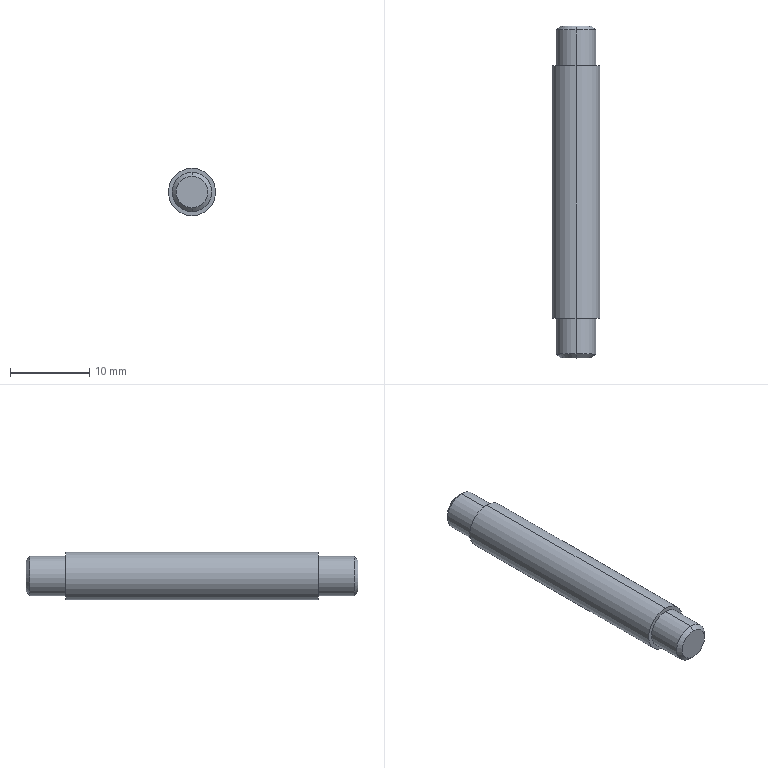Part | STEP file | Polyurethane roller shaft | 1 solid | 14 faces | box 6 x 42 x 6 mm | volume 1097 mm3 | cylinder 6 | cone 4 | plane 4 | commonest cylinder face diameters 5 x4 6 x2
STEP:
#1=CARTESIAN_POINT('',(0.,0.,0.));
#2=DIRECTION('',(0.,0.,1.));
#3=DIRECTION('',(1.,0.,0.));
#4=AXIS2_PLACEMENT_3D('',#1,#2,#3);
#5=CARTESIAN_POINT('',(0.,21.,2.));
#6=VERTEX_POINT('',#5);
#7=CARTESIAN_POINT('',(0.,21.,-2.));
#8=VERTEX_POINT('',#7);
#9=CARTESIAN_POINT('',(0.,21.,0.));
#10=DIRECTION('',(0.,1.,0.));
#11=DIRECTION('',(0.,0.,-1.));
#12=AXIS2_PLACEMENT_3D('',#9,#10,#11);
#13=CIRCLE('',#12,2.);
#14=CARTESIAN_POINT('',(0.,20.5,0.));
#15=DIRECTION('',(0.,-1.,0.));
#16=DIRECTION('',(0.,0.,-1.));
#17=AXIS2_PLACEMENT_3D('',#14,#15,#16);
#18=CONICAL_SURFACE('',#17,2.5,0.7854);
#19=CARTESIAN_POINT('',(6.283,-0.5));
#20=DIRECTION('',(-1.,0.));
#21=VECTOR('',#20,1.);
#22=LINE('',#19,#21);
#23=(GEOMETRIC_REPRESENTATION_CONTEXT(2)PARAMETRIC_REPRESENTATION_CONTEXT()REPRESENTATION_CONTEXT('',''));
#24=DEFINITIONAL_REPRESENTATION('',(#22),#23);
#25=PCURVE('',#18,#24);
#26=CARTESIAN_POINT('',(0.,21.,0.));
#27=DIRECTION('',(0.,-1.,0.));
#28=DIRECTION('',(0.,0.,-1.));
#29=AXIS2_PLACEMENT_3D('',#26,#27,#28);
#30=PLANE('',#29);
#31=CARTESIAN_POINT('',(2.,0.));
#32=CARTESIAN_POINT('',(2.,-3.464));
#33=CARTESIAN_POINT('',(-1.,-1.732));
#34=CARTESIAN_POINT('',(-4.,0.));
#35=CARTESIAN_POINT('',(-1.,1.732));
#36=CARTESIAN_POINT('',(2.,3.464));
#37=CARTESIAN_POINT('',(2.,0.));
#38=(BOUNDED_CURVE()B_SPLINE_CURVE(2,(#31,#32,#33,#34,#35,#36,#37),.UNSPECIFIED.,.T.,.F.)B_SPLINE_CURVE_WITH_KNOTS((1,2,2,2,2,1),(-2.094,0.,2.094,4.189,6.283,8.378),.UNSPECIFIED.)CURVE()GEOMETRIC_REPRESENTATION_ITEM()RATIONAL_B_SPLINE_CURVE((1.,0.5,1.,0.5,1.,0.5,1.))REPRESENTATION_ITEM(''));
#39=(GEOMETRIC_REPRESENTATION_CONTEXT(2)PARAMETRIC_REPRESENTATION_CONTEXT()REPRESENTATION_CONTEXT('',''));
#40=DEFINITIONAL_REPRESENTATION('',(#38),#39);
#41=PCURVE('',#30,#40);
#42=SURFACE_CURVE('',#13,(#25,#41),.PCURVE_S1.);
#43=EDGE_CURVE('',#6,#8,#42,.T.);
#44=ORIENTED_EDGE('',*,*,#43,.F.);
#45=CARTESIAN_POINT('',(0.,20.5,2.5));
#46=VERTEX_POINT('',#45);
#47=CARTESIAN_POINT('',(0.,20.5,2.5));
#48=DIRECTION('',(0.,-0.7071,0.7071));
#49=VECTOR('',#48,1.);
#50=LINE('',#47,#49);
#51=CARTESIAN_POINT('',(3.142,0.));
#52=DIRECTION('',(0.,1.));
#53=VECTOR('',#52,1.);
#54=LINE('',#51,#53);
#55=(GEOMETRIC_REPRESENTATION_CONTEXT(2)PARAMETRIC_REPRESENTATION_CONTEXT()REPRESENTATION_CONTEXT('',''));
#56=DEFINITIONAL_REPRESENTATION('',(#54),#55);
#57=PCURVE('',#18,#56);
#58=CARTESIAN_POINT('',(0.,20.5,0.));
#59=DIRECTION('',(0.,-1.,0.));
#60=DIRECTION('',(0.,0.,-1.));
#61=AXIS2_PLACEMENT_3D('',#58,#59,#60);
#62=CONICAL_SURFACE('',#61,2.5,0.7854);
#63=CARTESIAN_POINT('',(3.142,0.));
#64=DIRECTION('',(0.,1.));
#65=VECTOR('',#64,1.);
#66=LINE('',#63,#65);
#67=(GEOMETRIC_REPRESENTATION_CONTEXT(2)PARAMETRIC_REPRESENTATION_CONTEXT()REPRESENTATION_CONTEXT('',''));
#68=DEFINITIONAL_REPRESENTATION('',(#66),#67);
#69=PCURVE('',#62,#68);
#70=SURFACE_CURVE('',#50,(#57,#69),.PCURVE_S1.);
#71=EDGE_CURVE('',#6,#46,#70,.T.);
#72=ORIENTED_EDGE('',*,*,#71,.T.);
#73=CARTESIAN_POINT('',(0.,20.5,-2.5));
#74=VERTEX_POINT('',#73);
#75=CARTESIAN_POINT('',(0.,20.5,0.));
#76=DIRECTION('',(0.,-1.,0.));
#77=DIRECTION('',(0.,0.,-1.));
#78=AXIS2_PLACEMENT_3D('',#75,#76,#77);
#79=CIRCLE('',#78,2.5);
#80=CARTESIAN_POINT('',(0.,0.));
#81=DIRECTION('',(1.,0.));
#82=VECTOR('',#81,1.);
#83=LINE('',#80,#82);
#84=(GEOMETRIC_REPRESENTATION_CONTEXT(2)PARAMETRIC_REPRESENTATION_CONTEXT()REPRESENTATION_CONTEXT('',''));
#85=DEFINITIONAL_REPRESENTATION('',(#83),#84);
#86=PCURVE('',#18,#85);
#87=CARTESIAN_POINT('',(0.,-21.,0.));
#88=DIRECTION('',(0.,-1.,0.));
#89=DIRECTION('',(0.,0.,-1.));
#90=AXIS2_PLACEMENT_3D('',#87,#88,#89);
#91=CYLINDRICAL_SURFACE('',#90,2.5);
#92=CARTESIAN_POINT('',(0.,-41.5));
#93=DIRECTION('',(1.,0.));
#94=VECTOR('',#93,1.);
#95=LINE('',#92,#94);
#96=(GEOMETRIC_REPRESENTATION_CONTEXT(2)PARAMETRIC_REPRESENTATION_CONTEXT()REPRESENTATION_CONTEXT('',''));
#97=DEFINITIONAL_REPRESENTATION('',(#95),#96);
#98=PCURVE('',#91,#97);
#99=SURFACE_CURVE('',#79,(#86,#98),.PCURVE_S1.);
#100=EDGE_CURVE('',#74,#46,#99,.T.);
#101=ORIENTED_EDGE('',*,*,#100,.F.);
#102=CARTESIAN_POINT('',(0.,20.5,-2.5));
#103=DIRECTION('',(0.,-0.7071,-0.7071));
#104=VECTOR('',#103,1.);
#105=LINE('',#102,#104);
#106=CARTESIAN_POINT('',(0.,0.));
#107=DIRECTION('',(0.,1.));
#108=VECTOR('',#107,1.);
#109=LINE('',#106,#108);
#110=(GEOMETRIC_REPRESENTATION_CONTEXT(2)PARAMETRIC_REPRESENTATION_CONTEXT()REPRESENTATION_CONTEXT('',''));
#111=DEFINITIONAL_REPRESENTATION('',(#109),#110);
#112=PCURVE('',#18,#111);
#113=CARTESIAN_POINT('',(6.283,0.));
#114=DIRECTION('',(0.,1.));
#115=VECTOR('',#114,1.);
#116=LINE('',#113,#115);
#117=(GEOMETRIC_REPRESENTATION_CONTEXT(2)PARAMETRIC_REPRESENTATION_CONTEXT()REPRESENTATION_CONTEXT('',''));
#118=DEFINITIONAL_REPRESENTATION('',(#116),#117);
#119=PCURVE('',#62,#118);
#120=SURFACE_CURVE('',#105,(#112,#119),.PCURVE_S1.);
#121=EDGE_CURVE('',#8,#74,#120,.T.);
#122=ORIENTED_EDGE('',*,*,#121,.F.);
#123=EDGE_LOOP('',(#44,#72,#101,#122));
#124=FACE_BOUND('',#123,.T.);
#125=ADVANCED_FACE('',(#124),#18,.T.);
#126=CARTESIAN_POINT('',(0.,-21.,-2.));
#127=VERTEX_POINT('',#126);
#128=CARTESIAN_POINT('',(0.,-21.,2.));
#129=VERTEX_POINT('',#128);
#130=CARTESIAN_POINT('',(0.,-21.,0.));
#131=DIRECTION('',(0.,-1.,0.));
#132=DIRECTION('',(0.,0.,1.));
#133=AXIS2_PLACEMENT_3D('',#130,#131,#132);
#134=CIRCLE('',#133,2.);
#135=CARTESIAN_POINT('',(0.,-21.,0.));
#136=DIRECTION('',(0.,1.,0.));
#137=DIRECTION('',(0.,0.,1.));
#138=AXIS2_PLACEMENT_3D('',#135,#136,#137);
#139=CONICAL_SURFACE('',#138,2.,0.7854);
#140=CARTESIAN_POINT('',(6.283,0.));
#141=DIRECTION('',(-1.,0.));
#142=VECTOR('',#141,1.);
#143=LINE('',#140,#142);
#144=(GEOMETRIC_REPRESENTATION_CONTEXT(2)PARAMETRIC_REPRESENTATION_CONTEXT()REPRESENTATION_CONTEXT('',''));
#145=DEFINITIONAL_REPRESENTATION('',(#143),#144);
#146=PCURVE('',#139,#145);
#147=CARTESIAN_POINT('',(-2.5,-21.,0.));
#148=DIRECTION('',(0.,1.,0.));
#149=DIRECTION('',(0.,0.,1.));
#150=AXIS2_PLACEMENT_3D('',#147,#148,#149);
#151=PLANE('',#150);
#152=CARTESIAN_POINT('',(2.,2.5));
#153=CARTESIAN_POINT('',(2.,-0.9641));
#154=CARTESIAN_POINT('',(-1.,0.7679));
#155=CARTESIAN_POINT('',(-4.,2.5));
#156=CARTESIAN_POINT('',(-1.,4.232));
#157=CARTESIAN_POINT('',(2.,5.964));
#158=CARTESIAN_POINT('',(2.,2.5));
#159=(BOUNDED_CURVE()B_SPLINE_CURVE(2,(#152,#153,#154,#155,#156,#157,#158),.UNSPECIFIED.,.T.,.F.)B_SPLINE_CURVE_WITH_KNOTS((1,2,2,2,2,1),(-2.094,0.,2.094,4.189,6.283,8.378),.UNSPECIFIED.)CURVE()GEOMETRIC_REPRESENTATION_ITEM()RATIONAL_B_SPLINE_CURVE((1.,0.5,1.,0.5,1.,0.5,1.))REPRESENTATION_ITEM(''));
#160=(GEOMETRIC_REPRESENTATION_CONTEXT(2)PARAMETRIC_REPRESENTATION_CONTEXT()REPRESENTATION_CONTEXT('',''));
#161=DEFINITIONAL_REPRESENTATION('',(#159),#160);
#162=PCURVE('',#151,#161);
#163=SURFACE_CURVE('',#134,(#146,#162),.PCURVE_S1.);
#164=EDGE_CURVE('',#127,#129,#163,.T.);
#165=ORIENTED_EDGE('',*,*,#164,.F.);
#166=CARTESIAN_POINT('',(0.,-20.5,-2.5));
#167=VERTEX_POINT('',#166);
#168=CARTESIAN_POINT('',(0.,-21.,-2.));
#169=DIRECTION('',(0.,0.7071,-0.7071));
#170=VECTOR('',#169,1.);
#171=LINE('',#168,#170);
#172=CARTESIAN_POINT('',(3.142,0.));
#173=DIRECTION('',(0.,1.));
#174=VECTOR('',#173,1.);
#175=LINE('',#172,#174);
#176=(GEOMETRIC_REPRESENTATION_CONTEXT(2)PARAMETRIC_REPRESENTATION_CONTEXT()REPRESENTATION_CONTEXT('',''));
#177=DEFINITIONAL_REPRESENTATION('',(#175),#176);
#178=PCURVE('',#139,#177);
#179=CARTESIAN_POINT('',(0.,-21.,0.));
#180=DIRECTION('',(0.,1.,0.));
#181=DIRECTION('',(0.,0.,1.));
#182=AXIS2_PLACEMENT_3D('',#179,#180,#181);
#183=CONICAL_SURFACE('',#182,2.,0.7854);
#184=CARTESIAN_POINT('',(3.142,0.));
#185=DIRECTION('',(0.,1.));
#186=VECTOR('',#185,1.);
#187=LINE('',#184,#186);
#188=(GEOMETRIC_REPRESENTATION_CONTEXT(2)PARAMETRIC_REPRESENTATION_CONTEXT()REPRESENTATION_CONTEXT('',''));
#189=DEFINITIONAL_REPRESENTATION('',(#187),#188);
#190=PCURVE('',#183,#189);
#191=SURFACE_CURVE('',#171,(#178,#190),.PCURVE_S1.);
#192=EDGE_CURVE('',#127,#167,#191,.T.);
#193=ORIENTED_EDGE('',*,*,#192,.T.);
#194=CARTESIAN_POINT('',(0.,-20.5,2.5));
#195=VERTEX_POINT('',#194);
#196=CARTESIAN_POINT('',(0.,-20.5,0.));
#197=DIRECTION('',(0.,1.,0.));
#198=DIRECTION('',(0.,0.,1.));
#199=AXIS2_PLACEMENT_3D('',#196,#197,#198);
#200=CIRCLE('',#199,2.5);
#201=CARTESIAN_POINT('',(0.,0.5));
#202=DIRECTION('',(1.,0.));
#203=VECTOR('',#202,1.);
#204=LINE('',#201,#203);
#205=(GEOMETRIC_REPRESENTATION_CONTEXT(2)PARAMETRIC_REPRESENTATION_CONTEXT()REPRESENTATION_CONTEXT('',''));
#206=DEFINITIONAL_REPRESENTATION('',(#204),#205);
#207=PCURVE('',#139,#206);
#208=CARTESIAN_POINT('',(0.,-21.,0.));
#209=DIRECTION('',(0.,-1.,0.));
#210=DIRECTION('',(0.,0.,-1.));
#211=AXIS2_PLACEMENT_3D('',#208,#209,#210);
#212=CYLINDRICAL_SURFACE('',#211,2.5);
#213=CARTESIAN_POINT('',(3.142,-0.5));
#214=DIRECTION('',(-1.,0.));
#215=VECTOR('',#214,1.);
#216=LINE('',#213,#215);
#217=(GEOMETRIC_REPRESENTATION_CONTEXT(2)PARAMETRIC_REPRESENTATION_CONTEXT()REPRESENTATION_CONTEXT('',''));
#218=DEFINITIONAL_REPRESENTATION('',(#216),#217);
#219=PCURVE('',#212,#218);
#220=SURFACE_CURVE('',#200,(#207,#219),.PCURVE_S1.);
#221=EDGE_CURVE('',#195,#167,#220,.T.);
#222=ORIENTED_EDGE('',*,*,#221,.F.);
#223=CARTESIAN_POINT('',(0.,-21.,2.));
#224=DIRECTION('',(0.,0.7071,0.7071));
#225=VECTOR('',#224,1.);
#226=LINE('',#223,#225);
#227=CARTESIAN_POINT('',(0.,0.));
#228=DIRECTION('',(0.,1.));
#229=VECTOR('',#228,1.);
#230=LINE('',#227,#229);
#231=(GEOMETRIC_REPRESENTATION_CONTEXT(2)PARAMETRIC_REPRESENTATION_CONTEXT()REPRESENTATION_CONTEXT('',''));
#232=DEFINITIONAL_REPRESENTATION('',(#230),#231);
#233=PCURVE('',#139,#232);
#234=CARTESIAN_POINT('',(6.283,0.));
#235=DIRECTION('',(0.,1.));
#236=VECTOR('',#235,1.);
#237=LINE('',#234,#236);
#238=(GEOMETRIC_REPRESENTATION_CONTEXT(2)PARAMETRIC_REPRESENTATION_CONTEXT()REPRESENTATION_CONTEXT('',''));
#239=DEFINITIONAL_REPRESENTATION('',(#237),#238);
#240=PCURVE('',#183,#239);
#241=SURFACE_CURVE('',#226,(#233,#240),.PCURVE_S1.);
#242=EDGE_CURVE('',#129,#195,#241,.T.);
#243=ORIENTED_EDGE('',*,*,#242,.F.);
#244=EDGE_LOOP('',(#165,#193,#222,#243));
#245=FACE_BOUND('',#244,.T.);
#246=ADVANCED_FACE('',(#245),#139,.T.);
#247=CARTESIAN_POINT('',(0.,-16.,-2.5));
#248=VERTEX_POINT('',#247);
#249=CARTESIAN_POINT('',(0.,-16.,2.5));
#250=VERTEX_POINT('',#249);
#251=CARTESIAN_POINT('',(0.,-16.,0.));
#252=DIRECTION('',(0.,-1.,0.));
#253=DIRECTION('',(0.,0.,-1.));
#254=AXIS2_PLACEMENT_3D('',#251,#252,#253);
#255=CIRCLE('',#254,2.5);
#256=CARTESIAN_POINT('',(0.,-5.));
#257=DIRECTION('',(1.,0.));
#258=VECTOR('',#257,1.);
#259=LINE('',#256,#258);
#260=(GEOMETRIC_REPRESENTATION_CONTEXT(2)PARAMETRIC_REPRESENTATION_CONTEXT()REPRESENTATION_CONTEXT('',''));
#261=DEFINITIONAL_REPRESENTATION('',(#259),#260);
#262=PCURVE('',#212,#261);
#263=CARTESIAN_POINT('',(-3.,-16.,0.));
#264=DIRECTION('',(0.,1.,0.));
#265=DIRECTION('',(0.,0.,1.));
#266=AXIS2_PLACEMENT_3D('',#263,#264,#265);
#267=PLANE('',#266);
#268=CARTESIAN_POINT('',(-2.5,3.));
#269=CARTESIAN_POINT('',(-2.5,7.33));
#270=CARTESIAN_POINT('',(1.25,5.165));
#271=CARTESIAN_POINT('',(5.,3.));
#272=CARTESIAN_POINT('',(1.25,0.8349));
#273=CARTESIAN_POINT('',(-2.5,-1.33));
#274=CARTESIAN_POINT('',(-2.5,3.));
#275=(BOUNDED_CURVE()B_SPLINE_CURVE(2,(#268,#269,#270,#271,#272,#273,#274),.UNSPECIFIED.,.T.,.F.)B_SPLINE_CURVE_WITH_KNOTS((1,2,2,2,2,1),(-2.094,0.,2.094,4.189,6.283,8.378),.UNSPECIFIED.)CURVE()GEOMETRIC_REPRESENTATION_ITEM()RATIONAL_B_SPLINE_CURVE((1.,0.5,1.,0.5,1.,0.5,1.))REPRESENTATION_ITEM(''));
#276=(GEOMETRIC_REPRESENTATION_CONTEXT(2)PARAMETRIC_REPRESENTATION_CONTEXT()REPRESENTATION_CONTEXT('',''));
#277=DEFINITIONAL_REPRESENTATION('',(#275),#276);
#278=PCURVE('',#267,#277);
#279=SURFACE_CURVE('',#255,(#262,#278),.PCURVE_S1.);
#280=EDGE_CURVE('',#248,#250,#279,.T.);
#281=ORIENTED_EDGE('',*,*,#280,.T.);
#282=CARTESIAN_POINT('',(0.,-21.,2.5));
#283=DIRECTION('',(0.,-1.,0.));
#284=VECTOR('',#283,1.);
#285=LINE('',#282,#284);
#286=CARTESIAN_POINT('',(3.142,0.));
#287=DIRECTION('',(0.,1.));
#288=VECTOR('',#287,1.);
#289=LINE('',#286,#288);
#290=(GEOMETRIC_REPRESENTATION_CONTEXT(2)PARAMETRIC_REPRESENTATION_CONTEXT()REPRESENTATION_CONTEXT('',''));
#291=DEFINITIONAL_REPRESENTATION('',(#289),#290);
#292=PCURVE('',#212,#291);
#293=CARTESIAN_POINT('',(0.,-21.,0.));
#294=DIRECTION('',(0.,-1.,0.));
#295=DIRECTION('',(0.,0.,-1.));
#296=AXIS2_PLACEMENT_3D('',#293,#294,#295);
#297=CYLINDRICAL_SURFACE('',#296,2.5);
#298=CARTESIAN_POINT('',(3.142,0.));
#299=DIRECTION('',(0.,1.));
#300=VECTOR('',#299,1.);
#301=LINE('',#298,#300);
#302=(GEOMETRIC_REPRESENTATION_CONTEXT(2)PARAMETRIC_REPRESENTATION_CONTEXT()REPRESENTATION_CONTEXT('',''));
#303=DEFINITIONAL_REPRESENTATION('',(#301),#302);
#304=PCURVE('',#297,#303);
#305=SURFACE_CURVE('',#285,(#292,#304),.PCURVE_S1.);
#306=EDGE_CURVE('',#250,#195,#305,.T.);
#307=ORIENTED_EDGE('',*,*,#306,.T.);
#308=ORIENTED_EDGE('',*,*,#221,.T.);
#309=CARTESIAN_POINT('',(0.,-21.,-2.5));
#310=DIRECTION('',(0.,-1.,0.));
#311=VECTOR('',#310,1.);
#312=LINE('',#309,#311);
#313=CARTESIAN_POINT('',(0.,0.));
#314=DIRECTION('',(0.,1.));
#315=VECTOR('',#314,1.);
#316=LINE('',#313,#315);
#317=(GEOMETRIC_REPRESENTATION_CONTEXT(2)PARAMETRIC_REPRESENTATION_CONTEXT()REPRESENTATION_CONTEXT('',''));
#318=DEFINITIONAL_REPRESENTATION('',(#316),#317);
#319=PCURVE('',#212,#318);
#320=CARTESIAN_POINT('',(6.283,0.));
#321=DIRECTION('',(0.,1.));
#322=VECTOR('',#321,1.);
#323=LINE('',#320,#322);
#324=(GEOMETRIC_REPRESENTATION_CONTEXT(2)PARAMETRIC_REPRESENTATION_CONTEXT()REPRESENTATION_CONTEXT('',''));
#325=DEFINITIONAL_REPRESENTATION('',(#323),#324);
#326=PCURVE('',#297,#325);
#327=SURFACE_CURVE('',#312,(#319,#326),.PCURVE_S1.);
#328=EDGE_CURVE('',#248,#167,#327,.T.);
#329=ORIENTED_EDGE('',*,*,#328,.F.);
#330=EDGE_LOOP('',(#281,#307,#308,#329));
#331=FACE_BOUND('',#330,.T.);
#332=ADVANCED_FACE('',(#331),#212,.T.);
#333=CARTESIAN_POINT('',(0.,16.,-3.));
#334=VERTEX_POINT('',#333);
#335=CARTESIAN_POINT('',(0.,16.,3.));
#336=VERTEX_POINT('',#335);
#337=CARTESIAN_POINT('',(0.,16.,0.));
#338=DIRECTION('',(0.,-1.,0.));
#339=DIRECTION('',(0.,0.,-1.));
#340=AXIS2_PLACEMENT_3D('',#337,#338,#339);
#341=CIRCLE('',#340,3.);
#342=CARTESIAN_POINT('',(0.,-21.,0.));
#343=DIRECTION('',(0.,-1.,0.));
#344=DIRECTION('',(0.,0.,-1.));
#345=AXIS2_PLACEMENT_3D('',#342,#343,#344);
#346=CYLINDRICAL_SURFACE('',#345,3.);
#347=CARTESIAN_POINT('',(0.,-37.));
#348=DIRECTION('',(1.,0.));
#349=VECTOR('',#348,1.);
#350=LINE('',#347,#349);
#351=(GEOMETRIC_REPRESENTATION_CONTEXT(2)PARAMETRIC_REPRESENTATION_CONTEXT()REPRESENTATION_CONTEXT('',''));
#352=DEFINITIONAL_REPRESENTATION('',(#350),#351);
#353=PCURVE('',#346,#352);
#354=CARTESIAN_POINT('',(-2.5,16.,0.));
#355=DIRECTION('',(0.,-1.,0.));
#356=DIRECTION('',(0.,0.,-1.));
#357=AXIS2_PLACEMENT_3D('',#354,#355,#356);
#358=PLANE('',#357);
#359=CARTESIAN_POINT('',(0.,2.5));
#360=DIRECTION('',(1.,0.));
#361=AXIS2_PLACEMENT_2D('',#359,#360);
#362=CIRCLE('',#361,3.);
#363=(GEOMETRIC_REPRESENTATION_CONTEXT(2)PARAMETRIC_REPRESENTATION_CONTEXT()REPRESENTATION_CONTEXT('',''));
#364=DEFINITIONAL_REPRESENTATION('',(#362),#363);
#365=PCURVE('',#358,#364);
#366=SURFACE_CURVE('',#341,(#353,#365),.PCURVE_S1.);
#367=EDGE_CURVE('',#334,#336,#366,.T.);
#368=ORIENTED_EDGE('',*,*,#367,.T.);
#369=CARTESIAN_POINT('',(0.,-16.,3.));
#370=VERTEX_POINT('',#369);
#371=CARTESIAN_POINT('',(0.,-21.,3.));
#372=DIRECTION('',(0.,-1.,0.));
#373=VECTOR('',#372,1.);
#374=LINE('',#371,#373);
#375=CARTESIAN_POINT('',(3.142,0.));
#376=DIRECTION('',(0.,1.));
#377=VECTOR('',#376,1.);
#378=LINE('',#375,#377);
#379=(GEOMETRIC_REPRESENTATION_CONTEXT(2)PARAMETRIC_REPRESENTATION_CONTEXT()REPRESENTATION_CONTEXT('',''));
#380=DEFINITIONAL_REPRESENTATION('',(#378),#379);
#381=PCURVE('',#346,#380);
#382=CARTESIAN_POINT('',(0.,-21.,0.));
#383=DIRECTION('',(0.,-1.,0.));
#384=DIRECTION('',(0.,0.,-1.));
#385=AXIS2_PLACEMENT_3D('',#382,#383,#384);
#386=CYLINDRICAL_SURFACE('',#385,3.);
#387=CARTESIAN_POINT('',(3.142,0.));
#388=DIRECTION('',(0.,1.));
#389=VECTOR('',#388,1.);
#390=LINE('',#387,#389);
#391=(GEOMETRIC_REPRESENTATION_CONTEXT(2)PARAMETRIC_REPRESENTATION_CONTEXT()REPRESENTATION_CONTEXT('',''));
#392=DEFINITIONAL_REPRESENTATION('',(#390),#391);
#393=PCURVE('',#386,#392);
#394=SURFACE_CURVE('',#374,(#381,#393),.PCURVE_S1.);
#395=EDGE_CURVE('',#336,#370,#394,.T.);
#396=ORIENTED_EDGE('',*,*,#395,.T.);
#397=CARTESIAN_POINT('',(0.,-16.,-3.));
#398=VERTEX_POINT('',#397);
#399=CARTESIAN_POINT('',(0.,-16.,0.));
#400=DIRECTION('',(0.,-1.,0.));
#401=DIRECTION('',(0.,0.,-1.));
#402=AXIS2_PLACEMENT_3D('',#399,#400,#401);
#403=CIRCLE('',#402,3.);
#404=CARTESIAN_POINT('',(0.,-5.));
#405=DIRECTION('',(1.,0.));
#406=VECTOR('',#405,1.);
#407=LINE('',#404,#406);
#408=(GEOMETRIC_REPRESENTATION_CONTEXT(2)PARAMETRIC_REPRESENTATION_CONTEXT()REPRESENTATION_CONTEXT('',''));
#409=DEFINITIONAL_REPRESENTATION('',(#407),#408);
#410=PCURVE('',#346,#409);
#411=CARTESIAN_POINT('',(-3.,3.));
#412=CARTESIAN_POINT('',(-3.,8.196));
#413=CARTESIAN_POINT('',(1.5,5.598));
#414=CARTESIAN_POINT('',(6.,3.));
#415=CARTESIAN_POINT('',(1.5,0.4019));
#416=CARTESIAN_POINT('',(-3.,-2.196));
#417=CARTESIAN_POINT('',(-3.,3.));
#418=(BOUNDED_CURVE()B_SPLINE_CURVE(2,(#411,#412,#413,#414,#415,#416,#417),.UNSPECIFIED.,.T.,.F.)B_SPLINE_CURVE_WITH_KNOTS((1,2,2,2,2,1),(-2.094,0.,2.094,4.189,6.283,8.378),.UNSPECIFIED.)CURVE()GEOMETRIC_REPRESENTATION_ITEM()RATIONAL_B_SPLINE_CURVE((1.,0.5,1.,0.5,1.,0.5,1.))REPRESENTATION_ITEM(''));
#419=(GEOMETRIC_REPRESENTATION_CONTEXT(2)PARAMETRIC_REPRESENTATION_CONTEXT()REPRESENTATION_CONTEXT('',''));
#420=DEFINITIONAL_REPRESENTATION('',(#418),#419);
#421=PCURVE('',#267,#420);
#422=SURFACE_CURVE('',#403,(#410,#421),.PCURVE_S1.);
#423=EDGE_CURVE('',#398,#370,#422,.T.);
#424=ORIENTED_EDGE('',*,*,#423,.F.);
#425=CARTESIAN_POINT('',(0.,-21.,-3.));
#426=DIRECTION('',(0.,-1.,0.));
#427=VECTOR('',#426,1.);
#428=LINE('',#425,#427);
#429=CARTESIAN_POINT('',(0.,0.));
#430=DIRECTION('',(0.,1.));
#431=VECTOR('',#430,1.);
#432=LINE('',#429,#431);
#433=(GEOMETRIC_REPRESENTATION_CONTEXT(2)PARAMETRIC_REPRESENTATION_CONTEXT()REPRESENTATION_CONTEXT('',''));
#434=DEFINITIONAL_REPRESENTATION('',(#432),#433);
#435=PCURVE('',#346,#434);
#436=CARTESIAN_POINT('',(6.283,0.));
#437=DIRECTION('',(0.,1.));
#438=VECTOR('',#437,1.);
#439=LINE('',#436,#438);
#440=(GEOMETRIC_REPRESENTATION_CONTEXT(2)PARAMETRIC_REPRESENTATION_CONTEXT()REPRESENTATION_CONTEXT('',''));
#441=DEFINITIONAL_REPRESENTATION('',(#439),#440);
#442=PCURVE('',#386,#441);
#443=SURFACE_CURVE('',#428,(#435,#442),.PCURVE_S1.);
#444=EDGE_CURVE('',#334,#398,#443,.T.);
#445=ORIENTED_EDGE('',*,*,#444,.F.);
#446=EDGE_LOOP('',(#368,#396,#424,#445));
#447=FACE_BOUND('',#446,.T.);
#448=ADVANCED_FACE('',(#447),#346,.T.);
#449=ORIENTED_EDGE('',*,*,#100,.T.);
#450=CARTESIAN_POINT('',(0.,16.,2.5));
#451=VERTEX_POINT('',#450);
#452=CARTESIAN_POINT('',(0.,-21.,2.5));
#453=DIRECTION('',(0.,-1.,0.));
#454=VECTOR('',#453,1.);
#455=LINE('',#452,#454);
#456=CARTESIAN_POINT('',(3.142,0.));
#457=DIRECTION('',(0.,1.));
#458=VECTOR('',#457,1.);
#459=LINE('',#456,#458);
#460=(GEOMETRIC_REPRESENTATION_CONTEXT(2)PARAMETRIC_REPRESENTATION_CONTEXT()REPRESENTATION_CONTEXT('',''));
#461=DEFINITIONAL_REPRESENTATION('',(#459),#460);
#462=PCURVE('',#91,#461);
#463=CARTESIAN_POINT('',(0.,-21.,0.));
#464=DIRECTION('',(0.,-1.,0.));
#465=DIRECTION('',(0.,0.,-1.));
#466=AXIS2_PLACEMENT_3D('',#463,#464,#465);
#467=CYLINDRICAL_SURFACE('',#466,2.5);
#468=CARTESIAN_POINT('',(3.142,0.));
#469=DIRECTION('',(0.,1.));
#470=VECTOR('',#469,1.);
#471=LINE('',#468,#470);
#472=(GEOMETRIC_REPRESENTATION_CONTEXT(2)PARAMETRIC_REPRESENTATION_CONTEXT()REPRESENTATION_CONTEXT('',''));
#473=DEFINITIONAL_REPRESENTATION('',(#471),#472);
#474=PCURVE('',#467,#473);
#475=SURFACE_CURVE('',#455,(#462,#474),.PCURVE_S1.);
#476=EDGE_CURVE('',#46,#451,#475,.T.);
#477=ORIENTED_EDGE('',*,*,#476,.T.);
#478=CARTESIAN_POINT('',(0.,16.,-2.5));
#479=VERTEX_POINT('',#478);
#480=CARTESIAN_POINT('',(0.,16.,0.));
#481=DIRECTION('',(0.,-1.,0.));
#482=DIRECTION('',(0.,0.,-1.));
#483=AXIS2_PLACEMENT_3D('',#480,#481,#482);
#484=CIRCLE('',#483,2.5);
#485=CARTESIAN_POINT('',(0.,-37.));
#486=DIRECTION('',(1.,0.));
#487=VECTOR('',#486,1.);
#488=LINE('',#485,#487);
#489=(GEOMETRIC_REPRESENTATION_CONTEXT(2)PARAMETRIC_REPRESENTATION_CONTEXT()REPRESENTATION_CONTEXT('',''));
#490=DEFINITIONAL_REPRESENTATION('',(#488),#489);
#491=PCURVE('',#91,#490);
#492=CARTESIAN_POINT('',(0.,2.5));
#493=DIRECTION('',(1.,0.));
#494=AXIS2_PLACEMENT_2D('',#492,#493);
#495=CIRCLE('',#494,2.5);
#496=(GEOMETRIC_REPRESENTATION_CONTEXT(2)PARAMETRIC_REPRESENTATION_CONTEXT()REPRESENTATION_CONTEXT('',''));
#497=DEFINITIONAL_REPRESENTATION('',(#495),#496);
#498=PCURVE('',#358,#497);
#499=SURFACE_CURVE('',#484,(#491,#498),.PCURVE_S1.);
#500=EDGE_CURVE('',#479,#451,#499,.T.);
#501=ORIENTED_EDGE('',*,*,#500,.F.);
#502=CARTESIAN_POINT('',(0.,-21.,-2.5));
#503=DIRECTION('',(0.,-1.,0.));
#504=VECTOR('',#503,1.);
#505=LINE('',#502,#504);
#506=CARTESIAN_POINT('',(0.,0.));
#507=DIRECTION('',(0.,1.));
#508=VECTOR('',#507,1.);
#509=LINE('',#506,#508);
#510=(GEOMETRIC_REPRESENTATION_CONTEXT(2)PARAMETRIC_REPRESENTATION_CONTEXT()REPRESENTATION_CONTEXT('',''));
#511=DEFINITIONAL_REPRESENTATION('',(#509),#510);
#512=PCURVE('',#91,#511);
#513=CARTESIAN_POINT('',(6.283,0.));
#514=DIRECTION('',(0.,1.));
#515=VECTOR('',#514,1.);
#516=LINE('',#513,#515);
#517=(GEOMETRIC_REPRESENTATION_CONTEXT(2)PARAMETRIC_REPRESENTATION_CONTEXT()REPRESENTATION_CONTEXT('',''));
#518=DEFINITIONAL_REPRESENTATION('',(#516),#517);
#519=PCURVE('',#467,#518);
#520=SURFACE_CURVE('',#505,(#512,#519),.PCURVE_S1.);
#521=EDGE_CURVE('',#74,#479,#520,.T.);
#522=ORIENTED_EDGE('',*,*,#521,.F.);
#523=EDGE_LOOP('',(#449,#477,#501,#522));
#524=FACE_BOUND('',#523,.T.);
#525=ADVANCED_FACE('',(#524),#91,.T.);
#526=CARTESIAN_POINT('',(0.,-21.,0.));
#527=DIRECTION('',(0.,-1.,0.));
#528=DIRECTION('',(0.,0.,1.));
#529=AXIS2_PLACEMENT_3D('',#526,#527,#528);
#530=CIRCLE('',#529,2.);
#531=CARTESIAN_POINT('',(2.,2.5));
#532=CARTESIAN_POINT('',(2.,-0.9641));
#533=CARTESIAN_POINT('',(-1.,0.7679));
#534=CARTESIAN_POINT('',(-4.,2.5));
#535=CARTESIAN_POINT('',(-1.,4.232));
#536=CARTESIAN_POINT('',(2.,5.964));
#537=CARTESIAN_POINT('',(2.,2.5));
#538=(BOUNDED_CURVE()B_SPLINE_CURVE(2,(#531,#532,#533,#534,#535,#536,#537),.UNSPECIFIED.,.T.,.F.)B_SPLINE_CURVE_WITH_KNOTS((1,2,2,2,2,1),(-2.094,0.,2.094,4.189,6.283,8.378),.UNSPECIFIED.)CURVE()GEOMETRIC_REPRESENTATION_ITEM()RATIONAL_B_SPLINE_CURVE((1.,0.5,1.,0.5,1.,0.5,1.))REPRESENTATION_ITEM(''));
#539=(GEOMETRIC_REPRESENTATION_CONTEXT(2)PARAMETRIC_REPRESENTATION_CONTEXT()REPRESENTATION_CONTEXT('',''));
#540=DEFINITIONAL_REPRESENTATION('',(#538),#539);
#541=PCURVE('',#151,#540);
#542=CARTESIAN_POINT('',(6.283,0.));
#543=DIRECTION('',(-1.,0.));
#544=VECTOR('',#543,1.);
#545=LINE('',#542,#544);
#546=(GEOMETRIC_REPRESENTATION_CONTEXT(2)PARAMETRIC_REPRESENTATION_CONTEXT()REPRESENTATION_CONTEXT('',''));
#547=DEFINITIONAL_REPRESENTATION('',(#545),#546);
#548=PCURVE('',#183,#547);
#549=SURFACE_CURVE('',#530,(#541,#548),.PCURVE_S1.);
#550=EDGE_CURVE('',#129,#127,#549,.T.);
#551=ORIENTED_EDGE('',*,*,#550,.T.);
#552=ORIENTED_EDGE('',*,*,#164,.T.);
#553=EDGE_LOOP('',(#551,#552));
#554=FACE_BOUND('',#553,.T.);
#555=ADVANCED_FACE('',(#554),#151,.F.);
#556=CARTESIAN_POINT('',(0.,21.,0.));
#557=DIRECTION('',(0.,1.,0.));
#558=DIRECTION('',(0.,0.,-1.));
#559=AXIS2_PLACEMENT_3D('',#556,#557,#558);
#560=CIRCLE('',#559,2.);
#561=CARTESIAN_POINT('',(2.,0.));
#562=CARTESIAN_POINT('',(2.,-3.464));
#563=CARTESIAN_POINT('',(-1.,-1.732));
#564=CARTESIAN_POINT('',(-4.,0.));
#565=CARTESIAN_POINT('',(-1.,1.732));
#566=CARTESIAN_POINT('',(2.,3.464));
#567=CARTESIAN_POINT('',(2.,0.));
#568=(BOUNDED_CURVE()B_SPLINE_CURVE(2,(#561,#562,#563,#564,#565,#566,#567),.UNSPECIFIED.,.T.,.F.)B_SPLINE_CURVE_WITH_KNOTS((1,2,2,2,2,1),(-2.094,0.,2.094,4.189,6.283,8.378),.UNSPECIFIED.)CURVE()GEOMETRIC_REPRESENTATION_ITEM()RATIONAL_B_SPLINE_CURVE((1.,0.5,1.,0.5,1.,0.5,1.))REPRESENTATION_ITEM(''));
#569=(GEOMETRIC_REPRESENTATION_CONTEXT(2)PARAMETRIC_REPRESENTATION_CONTEXT()REPRESENTATION_CONTEXT('',''));
#570=DEFINITIONAL_REPRESENTATION('',(#568),#569);
#571=PCURVE('',#30,#570);
#572=CARTESIAN_POINT('',(6.283,-0.5));
#573=DIRECTION('',(-1.,0.));
#574=VECTOR('',#573,1.);
#575=LINE('',#572,#574);
#576=(GEOMETRIC_REPRESENTATION_CONTEXT(2)PARAMETRIC_REPRESENTATION_CONTEXT()REPRESENTATION_CONTEXT('',''));
#577=DEFINITIONAL_REPRESENTATION('',(#575),#576);
#578=PCURVE('',#62,#577);
#579=SURFACE_CURVE('',#560,(#571,#578),.PCURVE_S1.);
#580=EDGE_CURVE('',#8,#6,#579,.T.);
#581=ORIENTED_EDGE('',*,*,#580,.T.);
#582=ORIENTED_EDGE('',*,*,#43,.T.);
#583=EDGE_LOOP('',(#581,#582));
#584=FACE_BOUND('',#583,.T.);
#585=ADVANCED_FACE('',(#584),#30,.F.);
#586=ORIENTED_EDGE('',*,*,#476,.F.);
#587=CARTESIAN_POINT('',(0.,20.5,0.));
#588=DIRECTION('',(0.,-1.,0.));
#589=DIRECTION('',(0.,0.,-1.));
#590=AXIS2_PLACEMENT_3D('',#587,#588,#589);
#591=CIRCLE('',#590,2.5);
#592=CARTESIAN_POINT('',(0.,-41.5));
#593=DIRECTION('',(1.,0.));
#594=VECTOR('',#593,1.);
#595=LINE('',#592,#594);
#596=(GEOMETRIC_REPRESENTATION_CONTEXT(2)PARAMETRIC_REPRESENTATION_CONTEXT()REPRESENTATION_CONTEXT('',''));
#597=DEFINITIONAL_REPRESENTATION('',(#595),#596);
#598=PCURVE('',#467,#597);
#599=CARTESIAN_POINT('',(0.,0.));
#600=DIRECTION('',(1.,0.));
#601=VECTOR('',#600,1.);
#602=LINE('',#599,#601);
#603=(GEOMETRIC_REPRESENTATION_CONTEXT(2)PARAMETRIC_REPRESENTATION_CONTEXT()REPRESENTATION_CONTEXT('',''));
#604=DEFINITIONAL_REPRESENTATION('',(#602),#603);
#605=PCURVE('',#62,#604);
#606=SURFACE_CURVE('',#591,(#598,#605),.PCURVE_S1.);
#607=EDGE_CURVE('',#46,#74,#606,.T.);
#608=ORIENTED_EDGE('',*,*,#607,.T.);
#609=ORIENTED_EDGE('',*,*,#521,.T.);
#610=CARTESIAN_POINT('',(0.,16.,0.));
#611=DIRECTION('',(0.,-1.,0.));
#612=DIRECTION('',(0.,0.,-1.));
#613=AXIS2_PLACEMENT_3D('',#610,#611,#612);
#614=CIRCLE('',#613,2.5);
#615=CARTESIAN_POINT('',(0.,-37.));
#616=DIRECTION('',(1.,0.));
#617=VECTOR('',#616,1.);
#618=LINE('',#615,#617);
#619=(GEOMETRIC_REPRESENTATION_CONTEXT(2)PARAMETRIC_REPRESENTATION_CONTEXT()REPRESENTATION_CONTEXT('',''));
#620=DEFINITIONAL_REPRESENTATION('',(#618),#619);
#621=PCURVE('',#467,#620);
#622=CARTESIAN_POINT('',(0.,2.5));
#623=DIRECTION('',(1.,0.));
#624=AXIS2_PLACEMENT_2D('',#622,#623);
#625=CIRCLE('',#624,2.5);
#626=(GEOMETRIC_REPRESENTATION_CONTEXT(2)PARAMETRIC_REPRESENTATION_CONTEXT()REPRESENTATION_CONTEXT('',''));
#627=DEFINITIONAL_REPRESENTATION('',(#625),#626);
#628=PCURVE('',#358,#627);
#629=SURFACE_CURVE('',#614,(#621,#628),.PCURVE_S1.);
#630=EDGE_CURVE('',#451,#479,#629,.T.);
#631=ORIENTED_EDGE('',*,*,#630,.F.);
#632=EDGE_LOOP('',(#586,#608,#609,#631));
#633=FACE_BOUND('',#632,.T.);
#634=ADVANCED_FACE('',(#633),#467,.T.);
#635=ORIENTED_EDGE('',*,*,#367,.F.);
#636=CARTESIAN_POINT('',(0.,16.,0.));
#637=DIRECTION('',(0.,-1.,0.));
#638=DIRECTION('',(0.,0.,-1.));
#639=AXIS2_PLACEMENT_3D('',#636,#637,#638);
#640=CIRCLE('',#639,3.);
#641=CARTESIAN_POINT('',(0.,2.5));
#642=DIRECTION('',(1.,0.));
#643=AXIS2_PLACEMENT_2D('',#641,#642);
#644=CIRCLE('',#643,3.);
#645=(GEOMETRIC_REPRESENTATION_CONTEXT(2)PARAMETRIC_REPRESENTATION_CONTEXT()REPRESENTATION_CONTEXT('',''));
#646=DEFINITIONAL_REPRESENTATION('',(#644),#645);
#647=PCURVE('',#358,#646);
#648=CARTESIAN_POINT('',(0.,-37.));
#649=DIRECTION('',(1.,0.));
#650=VECTOR('',#649,1.);
#651=LINE('',#648,#650);
#652=(GEOMETRIC_REPRESENTATION_CONTEXT(2)PARAMETRIC_REPRESENTATION_CONTEXT()REPRESENTATION_CONTEXT('',''));
#653=DEFINITIONAL_REPRESENTATION('',(#651),#652);
#654=PCURVE('',#386,#653);
#655=SURFACE_CURVE('',#640,(#647,#654),.PCURVE_S1.);
#656=EDGE_CURVE('',#336,#334,#655,.T.);
#657=ORIENTED_EDGE('',*,*,#656,.F.);
#658=EDGE_LOOP('',(#635,#657));
#659=FACE_BOUND('',#658,.T.);
#660=ORIENTED_EDGE('',*,*,#500,.T.);
#661=ORIENTED_EDGE('',*,*,#630,.T.);
#662=EDGE_LOOP('',(#660,#661));
#663=FACE_BOUND('',#662,.T.);
#664=ADVANCED_FACE('',(#659,#663),#358,.F.);
#665=ORIENTED_EDGE('',*,*,#395,.F.);
#666=ORIENTED_EDGE('',*,*,#656,.T.);
#667=ORIENTED_EDGE('',*,*,#444,.T.);
#668=CARTESIAN_POINT('',(0.,-16.,0.));
#669=DIRECTION('',(0.,-1.,0.));
#670=DIRECTION('',(0.,0.,-1.));
#671=AXIS2_PLACEMENT_3D('',#668,#669,#670);
#672=CIRCLE('',#671,3.);
#673=CARTESIAN_POINT('',(0.,-5.));
#674=DIRECTION('',(1.,0.));
#675=VECTOR('',#674,1.);
#676=LINE('',#673,#675);
#677=(GEOMETRIC_REPRESENTATION_CONTEXT(2)PARAMETRIC_REPRESENTATION_CONTEXT()REPRESENTATION_CONTEXT('',''));
#678=DEFINITIONAL_REPRESENTATION('',(#676),#677);
#679=PCURVE('',#386,#678);
#680=CARTESIAN_POINT('',(-3.,3.));
#681=CARTESIAN_POINT('',(-3.,8.196));
#682=CARTESIAN_POINT('',(1.5,5.598));
#683=CARTESIAN_POINT('',(6.,3.));
#684=CARTESIAN_POINT('',(1.5,0.4019));
#685=CARTESIAN_POINT('',(-3.,-2.196));
#686=CARTESIAN_POINT('',(-3.,3.));
#687=(BOUNDED_CURVE()B_SPLINE_CURVE(2,(#680,#681,#682,#683,#684,#685,#686),.UNSPECIFIED.,.T.,.F.)B_SPLINE_CURVE_WITH_KNOTS((1,2,2,2,2,1),(-2.094,0.,2.094,4.189,6.283,8.378),.UNSPECIFIED.)CURVE()GEOMETRIC_REPRESENTATION_ITEM()RATIONAL_B_SPLINE_CURVE((1.,0.5,1.,0.5,1.,0.5,1.))REPRESENTATION_ITEM(''));
#688=(GEOMETRIC_REPRESENTATION_CONTEXT(2)PARAMETRIC_REPRESENTATION_CONTEXT()REPRESENTATION_CONTEXT('',''));
#689=DEFINITIONAL_REPRESENTATION('',(#687),#688);
#690=PCURVE('',#267,#689);
#691=SURFACE_CURVE('',#672,(#679,#690),.PCURVE_S1.);
#692=EDGE_CURVE('',#370,#398,#691,.T.);
#693=ORIENTED_EDGE('',*,*,#692,.F.);
#694=EDGE_LOOP('',(#665,#666,#667,#693));
#695=FACE_BOUND('',#694,.T.);
#696=ADVANCED_FACE('',(#695),#386,.T.);
#697=ORIENTED_EDGE('',*,*,#280,.F.);
#698=CARTESIAN_POINT('',(0.,-16.,0.));
#699=DIRECTION('',(0.,-1.,0.));
#700=DIRECTION('',(0.,0.,-1.));
#701=AXIS2_PLACEMENT_3D('',#698,#699,#700);
#702=CIRCLE('',#701,2.5);
#703=CARTESIAN_POINT('',(-2.5,3.));
#704=CARTESIAN_POINT('',(-2.5,7.33));
#705=CARTESIAN_POINT('',(1.25,5.165));
#706=CARTESIAN_POINT('',(5.,3.));
#707=CARTESIAN_POINT('',(1.25,0.8349));
#708=CARTESIAN_POINT('',(-2.5,-1.33));
#709=CARTESIAN_POINT('',(-2.5,3.));
#710=(BOUNDED_CURVE()B_SPLINE_CURVE(2,(#703,#704,#705,#706,#707,#708,#709),.UNSPECIFIED.,.T.,.F.)B_SPLINE_CURVE_WITH_KNOTS((1,2,2,2,2,1),(-2.094,0.,2.094,4.189,6.283,8.378),.UNSPECIFIED.)CURVE()GEOMETRIC_REPRESENTATION_ITEM()RATIONAL_B_SPLINE_CURVE((1.,0.5,1.,0.5,1.,0.5,1.))REPRESENTATION_ITEM(''));
#711=(GEOMETRIC_REPRESENTATION_CONTEXT(2)PARAMETRIC_REPRESENTATION_CONTEXT()REPRESENTATION_CONTEXT('',''));
#712=DEFINITIONAL_REPRESENTATION('',(#710),#711);
#713=PCURVE('',#267,#712);
#714=CARTESIAN_POINT('',(0.,-5.));
#715=DIRECTION('',(1.,0.));
#716=VECTOR('',#715,1.);
#717=LINE('',#714,#716);
#718=(GEOMETRIC_REPRESENTATION_CONTEXT(2)PARAMETRIC_REPRESENTATION_CONTEXT()REPRESENTATION_CONTEXT('',''));
#719=DEFINITIONAL_REPRESENTATION('',(#717),#718);
#720=PCURVE('',#297,#719);
#721=SURFACE_CURVE('',#702,(#713,#720),.PCURVE_S1.);
#722=EDGE_CURVE('',#250,#248,#721,.T.);
#723=ORIENTED_EDGE('',*,*,#722,.F.);
#724=EDGE_LOOP('',(#697,#723));
#725=FACE_BOUND('',#724,.T.);
#726=ORIENTED_EDGE('',*,*,#423,.T.);
#727=ORIENTED_EDGE('',*,*,#692,.T.);
#728=EDGE_LOOP('',(#726,#727));
#729=FACE_BOUND('',#728,.T.);
#730=ADVANCED_FACE('',(#725,#729),#267,.F.);
#731=ORIENTED_EDGE('',*,*,#306,.F.);
#732=ORIENTED_EDGE('',*,*,#722,.T.);
#733=ORIENTED_EDGE('',*,*,#328,.T.);
#734=CARTESIAN_POINT('',(0.,-20.5,0.));
#735=DIRECTION('',(0.,1.,0.));
#736=DIRECTION('',(0.,0.,1.));
#737=AXIS2_PLACEMENT_3D('',#734,#735,#736);
#738=CIRCLE('',#737,2.5);
#739=CARTESIAN_POINT('',(9.425,-0.5));
#740=DIRECTION('',(-1.,0.));
#741=VECTOR('',#740,1.);
#742=LINE('',#739,#741);
#743=(GEOMETRIC_REPRESENTATION_CONTEXT(2)PARAMETRIC_REPRESENTATION_CONTEXT()REPRESENTATION_CONTEXT('',''));
#744=DEFINITIONAL_REPRESENTATION('',(#742),#743);
#745=PCURVE('',#297,#744);
#746=CARTESIAN_POINT('',(0.,0.5));
#747=DIRECTION('',(1.,0.));
#748=VECTOR('',#747,1.);
#749=LINE('',#746,#748);
#750=(GEOMETRIC_REPRESENTATION_CONTEXT(2)PARAMETRIC_REPRESENTATION_CONTEXT()REPRESENTATION_CONTEXT('',''));
#751=DEFINITIONAL_REPRESENTATION('',(#749),#750);
#752=PCURVE('',#183,#751);
#753=SURFACE_CURVE('',#738,(#745,#752),.PCURVE_S1.);
#754=EDGE_CURVE('',#167,#195,#753,.T.);
#755=ORIENTED_EDGE('',*,*,#754,.T.);
#756=EDGE_LOOP('',(#731,#732,#733,#755));
#757=FACE_BOUND('',#756,.T.);
#758=ADVANCED_FACE('',(#757),#297,.T.);
#759=ORIENTED_EDGE('',*,*,#192,.F.);
#760=ORIENTED_EDGE('',*,*,#550,.F.);
#761=ORIENTED_EDGE('',*,*,#242,.T.);
#762=ORIENTED_EDGE('',*,*,#754,.F.);
#763=EDGE_LOOP('',(#759,#760,#761,#762));
#764=FACE_BOUND('',#763,.T.);
#765=ADVANCED_FACE('',(#764),#183,.T.);
#766=ORIENTED_EDGE('',*,*,#71,.F.);
#767=ORIENTED_EDGE('',*,*,#580,.F.);
#768=ORIENTED_EDGE('',*,*,#121,.T.);
#769=ORIENTED_EDGE('',*,*,#607,.F.);
#770=EDGE_LOOP('',(#766,#767,#768,#769));
#771=FACE_BOUND('',#770,.T.);
#772=ADVANCED_FACE('',(#771),#62,.T.);
#773=CLOSED_SHELL('',(#125,#246,#332,#448,#525,#555,#585,#634,#664,#696,#730,#758,#765,#772));
#774=MANIFOLD_SOLID_BREP('',#773);
#775=(LENGTH_UNIT()NAMED_UNIT(*)SI_UNIT(.MILLI.,.METRE.));
#776=UNCERTAINTY_MEASURE_WITH_UNIT(LENGTH_MEASURE(0.0000001),#775,'','');
#777=(NAMED_UNIT(*)PLANE_ANGLE_UNIT()SI_UNIT($,.RADIAN.));
#778=(NAMED_UNIT(*)SI_UNIT($,.STERADIAN.)SOLID_ANGLE_UNIT());
#779=(GEOMETRIC_REPRESENTATION_CONTEXT(3)GLOBAL_UNCERTAINTY_ASSIGNED_CONTEXT((#776))GLOBAL_UNIT_ASSIGNED_CONTEXT((#775,#777,#778))REPRESENTATION_CONTEXT('',''));
#780=ADVANCED_BREP_SHAPE_REPRESENTATION('',(#4,#774),#779);